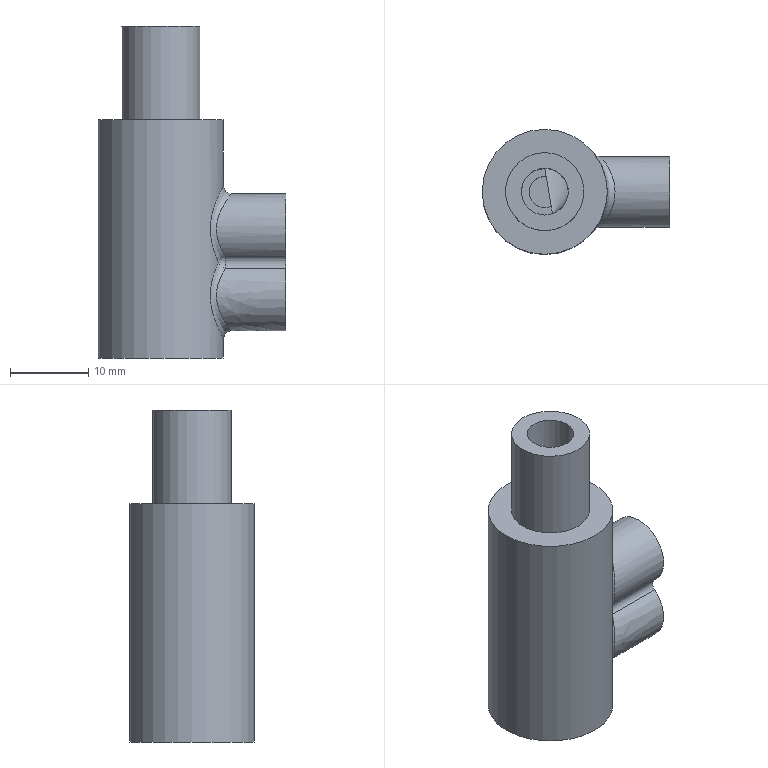Part | STEP file | 1-73.1 | 1 solid | 22 faces | box 24 x 16 x 42.5 mm | volume 6373 mm3 | cylinder 9 | plane 8 | spline 3 | sphere 2 | commonest cylinder face diameters 6 x3 2 x2 4 x1 9 x1 10 x1 16 x1